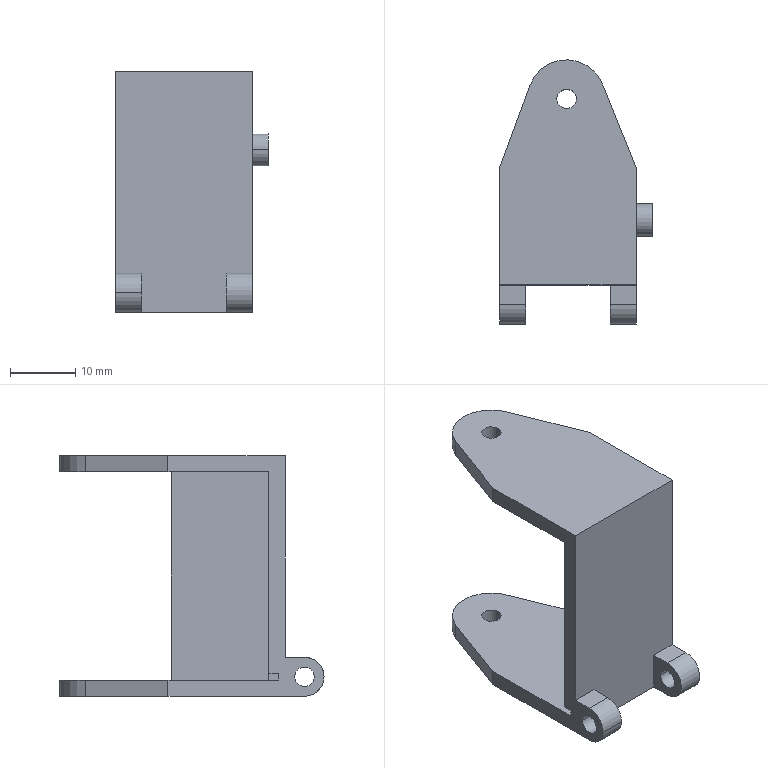Part | SolidWorks | features BaseBody 1 | 1 solid | 37 faces | box 23.5 x 40.616 x 37 mm | volume 6167 mm3 | plane 21 | cylinder 16 | commonest cylinder face diameters 3 x8 6 x3 5 x2 12 x2 8 x1
STEP:
#1=CARTESIAN_POINT('',(23.5,12.5,25.));
#2=VERTEX_POINT('',#1);
#3=CARTESIAN_POINT('',(23.5,7.5,25.));
#4=VERTEX_POINT('',#3);
#5=CARTESIAN_POINT('',(23.5,10.,25.));
#6=DIRECTION('',(1.,0.,0.));
#7=DIRECTION('',(0.,1.,0.));
#8=AXIS2_PLACEMENT_3D('',#5,#6,#7);
#9=CIRCLE('',#8,2.5);
#10=EDGE_CURVE('',#2,#4,#9,.T.);
#11=ORIENTED_EDGE('',*,*,#10,.F.);
#12=CARTESIAN_POINT('',(21.,12.5,25.));
#13=VERTEX_POINT('',#12);
#14=CARTESIAN_POINT('',(23.5,12.5,25.));
#15=DIRECTION('',(-1.,0.,0.));
#16=VECTOR('',#15,1000.);
#17=LINE('',#14,#16);
#18=EDGE_CURVE('',#2,#13,#17,.T.);
#19=ORIENTED_EDGE('',*,*,#18,.T.);
#20=CARTESIAN_POINT('',(21.,7.5,25.));
#21=VERTEX_POINT('',#20);
#22=CARTESIAN_POINT('',(21.,10.,25.));
#23=DIRECTION('',(1.,0.,0.));
#24=DIRECTION('',(0.,-1.,0.));
#25=AXIS2_PLACEMENT_3D('',#22,#23,#24);
#26=CIRCLE('',#25,2.5);
#27=EDGE_CURVE('',#13,#21,#26,.T.);
#28=ORIENTED_EDGE('',*,*,#27,.T.);
#29=CARTESIAN_POINT('',(23.5,7.5,25.));
#30=DIRECTION('',(-1.,0.,0.));
#31=VECTOR('',#30,1000.);
#32=LINE('',#29,#31);
#33=EDGE_CURVE('',#4,#21,#32,.T.);
#34=ORIENTED_EDGE('',*,*,#33,.F.);
#35=EDGE_LOOP('',(#11,#19,#28,#34));
#36=FACE_OUTER_BOUND('',#35,.T.);
#37=CARTESIAN_POINT('',(23.5,10.,25.));
#38=DIRECTION('',(-1.,0.,0.));
#39=DIRECTION('',(0.,-1.,0.));
#40=AXIS2_PLACEMENT_3D('',#37,#38,#39);
#41=CYLINDRICAL_SURFACE('',#40,2.5);
#42=ADVANCED_FACE('',(#36),#41,.T.);
#43=CARTESIAN_POINT('',(8.795,28.616,37.));
#44=VERTEX_POINT('',#43);
#45=CARTESIAN_POINT('',(11.795,28.616,37.));
#46=VERTEX_POINT('',#45);
#47=CARTESIAN_POINT('',(10.295,28.616,37.));
#48=DIRECTION('',(0.,0.,1.));
#49=DIRECTION('',(1.,0.,0.));
#50=AXIS2_PLACEMENT_3D('',#47,#48,#49);
#51=CIRCLE('',#50,1.5);
#52=EDGE_CURVE('',#44,#46,#51,.T.);
#53=ORIENTED_EDGE('',*,*,#52,.T.);
#54=CARTESIAN_POINT('',(11.795,28.616,34.5));
#55=VERTEX_POINT('',#54);
#56=CARTESIAN_POINT('',(11.795,28.616,43.));
#57=DIRECTION('',(0.,0.,-1.));
#58=VECTOR('',#57,1000.);
#59=LINE('',#56,#58);
#60=EDGE_CURVE('',#46,#55,#59,.T.);
#61=ORIENTED_EDGE('',*,*,#60,.T.);
#62=CARTESIAN_POINT('',(8.795,28.616,34.5));
#63=VERTEX_POINT('',#62);
#64=CARTESIAN_POINT('',(10.295,28.616,34.5));
#65=DIRECTION('',(0.,0.,1.));
#66=DIRECTION('',(1.,0.,0.));
#67=AXIS2_PLACEMENT_3D('',#64,#65,#66);
#68=CIRCLE('',#67,1.5);
#69=EDGE_CURVE('',#63,#55,#68,.T.);
#70=ORIENTED_EDGE('',*,*,#69,.F.);
#71=CARTESIAN_POINT('',(8.795,28.616,43.));
#72=DIRECTION('',(0.,0.,-1.));
#73=VECTOR('',#72,1000.);
#74=LINE('',#71,#73);
#75=EDGE_CURVE('',#44,#63,#74,.T.);
#76=ORIENTED_EDGE('',*,*,#75,.F.);
#77=EDGE_LOOP('',(#53,#61,#70,#76));
#78=FACE_OUTER_BOUND('',#77,.T.);
#79=CARTESIAN_POINT('',(10.295,28.616,43.));
#80=DIRECTION('',(0.,0.,-1.));
#81=DIRECTION('',(-1.,0.,0.));
#82=AXIS2_PLACEMENT_3D('',#79,#80,#81);
#83=CYLINDRICAL_SURFACE('',#82,1.5);
#84=ADVANCED_FACE('',(#78),#83,.F.);
#85=CARTESIAN_POINT('',(8.795,28.616,2.5));
#86=VERTEX_POINT('',#85);
#87=CARTESIAN_POINT('',(11.795,28.616,2.5));
#88=VERTEX_POINT('',#87);
#89=CARTESIAN_POINT('',(10.295,28.616,2.5));
#90=DIRECTION('',(0.,0.,1.));
#91=DIRECTION('',(1.,0.,0.));
#92=AXIS2_PLACEMENT_3D('',#89,#90,#91);
#93=CIRCLE('',#92,1.5);
#94=EDGE_CURVE('',#86,#88,#93,.T.);
#95=ORIENTED_EDGE('',*,*,#94,.T.);
#96=CARTESIAN_POINT('',(11.795,28.616,0.));
#97=VERTEX_POINT('',#96);
#98=CARTESIAN_POINT('',(11.795,28.616,43.));
#99=DIRECTION('',(0.,0.,-1.));
#100=VECTOR('',#99,1000.);
#101=LINE('',#98,#100);
#102=EDGE_CURVE('',#88,#97,#101,.T.);
#103=ORIENTED_EDGE('',*,*,#102,.T.);
#104=CARTESIAN_POINT('',(8.795,28.616,0.));
#105=VERTEX_POINT('',#104);
#106=CARTESIAN_POINT('',(10.295,28.616,0.));
#107=DIRECTION('',(0.,0.,-1.));
#108=DIRECTION('',(-1.,0.,0.));
#109=AXIS2_PLACEMENT_3D('',#106,#107,#108);
#110=CIRCLE('',#109,1.5);
#111=EDGE_CURVE('',#97,#105,#110,.T.);
#112=ORIENTED_EDGE('',*,*,#111,.T.);
#113=CARTESIAN_POINT('',(8.795,28.616,43.));
#114=DIRECTION('',(0.,0.,-1.));
#115=VECTOR('',#114,1000.);
#116=LINE('',#113,#115);
#117=EDGE_CURVE('',#86,#105,#116,.T.);
#118=ORIENTED_EDGE('',*,*,#117,.F.);
#119=EDGE_LOOP('',(#95,#103,#112,#118));
#120=FACE_OUTER_BOUND('',#119,.T.);
#121=CARTESIAN_POINT('',(10.295,28.616,43.));
#122=DIRECTION('',(0.,0.,-1.));
#123=DIRECTION('',(-1.,0.,0.));
#124=AXIS2_PLACEMENT_3D('',#121,#122,#123);
#125=CYLINDRICAL_SURFACE('',#124,1.5);
#126=ADVANCED_FACE('',(#120),#125,.F.);
#127=CARTESIAN_POINT('',(17.,-1.5,3.));
#128=VERTEX_POINT('',#127);
#129=CARTESIAN_POINT('',(17.,-4.5,3.));
#130=VERTEX_POINT('',#129);
#131=CARTESIAN_POINT('',(17.,-3.,3.));
#132=DIRECTION('',(-1.,0.,0.));
#133=DIRECTION('',(0.,-1.,0.));
#134=AXIS2_PLACEMENT_3D('',#131,#132,#133);
#135=CIRCLE('',#134,1.5);
#136=EDGE_CURVE('',#128,#130,#135,.T.);
#137=ORIENTED_EDGE('',*,*,#136,.T.);
#138=CARTESIAN_POINT('',(21.,-4.5,3.));
#139=VERTEX_POINT('',#138);
#140=CARTESIAN_POINT('',(17.,-4.5,3.));
#141=DIRECTION('',(1.,0.,0.));
#142=VECTOR('',#141,1000.);
#143=LINE('',#140,#142);
#144=EDGE_CURVE('',#130,#139,#143,.T.);
#145=ORIENTED_EDGE('',*,*,#144,.T.);
#146=CARTESIAN_POINT('',(21.,-1.5,3.));
#147=VERTEX_POINT('',#146);
#148=CARTESIAN_POINT('',(21.,-3.,3.));
#149=DIRECTION('',(-1.,0.,0.));
#150=DIRECTION('',(0.,-1.,0.));
#151=AXIS2_PLACEMENT_3D('',#148,#149,#150);
#152=CIRCLE('',#151,1.5);
#153=EDGE_CURVE('',#147,#139,#152,.T.);
#154=ORIENTED_EDGE('',*,*,#153,.F.);
#155=CARTESIAN_POINT('',(17.,-1.5,3.));
#156=DIRECTION('',(1.,0.,0.));
#157=VECTOR('',#156,1000.);
#158=LINE('',#155,#157);
#159=EDGE_CURVE('',#128,#147,#158,.T.);
#160=ORIENTED_EDGE('',*,*,#159,.F.);
#161=EDGE_LOOP('',(#137,#145,#154,#160));
#162=FACE_OUTER_BOUND('',#161,.T.);
#163=CARTESIAN_POINT('',(17.,-3.,3.));
#164=DIRECTION('',(1.,0.,0.));
#165=DIRECTION('',(0.,1.,0.));
#166=AXIS2_PLACEMENT_3D('',#163,#164,#165);
#167=CYLINDRICAL_SURFACE('',#166,1.5);
#168=ADVANCED_FACE('',(#162),#167,.F.);
#169=CARTESIAN_POINT('',(4.,-1.5,3.));
#170=VERTEX_POINT('',#169);
#171=CARTESIAN_POINT('',(4.,-4.5,3.));
#172=VERTEX_POINT('',#171);
#173=CARTESIAN_POINT('',(4.,-3.,3.));
#174=DIRECTION('',(-1.,0.,0.));
#175=DIRECTION('',(0.,-1.,0.));
#176=AXIS2_PLACEMENT_3D('',#173,#174,#175);
#177=CIRCLE('',#176,1.5);
#178=EDGE_CURVE('',#170,#172,#177,.T.);
#179=ORIENTED_EDGE('',*,*,#178,.F.);
#180=CARTESIAN_POINT('',(0.,-1.5,3.));
#181=VERTEX_POINT('',#180);
#182=CARTESIAN_POINT('',(4.,-1.5,3.));
#183=DIRECTION('',(-1.,0.,0.));
#184=VECTOR('',#183,1000.);
#185=LINE('',#182,#184);
#186=EDGE_CURVE('',#170,#181,#185,.T.);
#187=ORIENTED_EDGE('',*,*,#186,.T.);
#188=CARTESIAN_POINT('',(0.,-4.5,3.));
#189=VERTEX_POINT('',#188);
#190=CARTESIAN_POINT('',(0.,-3.,3.));
#191=DIRECTION('',(-1.,0.,0.));
#192=DIRECTION('',(0.,-1.,0.));
#193=AXIS2_PLACEMENT_3D('',#190,#191,#192);
#194=CIRCLE('',#193,1.5);
#195=EDGE_CURVE('',#181,#189,#194,.T.);
#196=ORIENTED_EDGE('',*,*,#195,.T.);
#197=CARTESIAN_POINT('',(4.,-4.5,3.));
#198=DIRECTION('',(-1.,0.,0.));
#199=VECTOR('',#198,1000.);
#200=LINE('',#197,#199);
#201=EDGE_CURVE('',#172,#189,#200,.T.);
#202=ORIENTED_EDGE('',*,*,#201,.F.);
#203=EDGE_LOOP('',(#179,#187,#196,#202));
#204=FACE_OUTER_BOUND('',#203,.T.);
#205=CARTESIAN_POINT('',(4.,-3.,3.));
#206=DIRECTION('',(-1.,0.,0.));
#207=DIRECTION('',(0.,-1.,0.));
#208=AXIS2_PLACEMENT_3D('',#205,#206,#207);
#209=CYLINDRICAL_SURFACE('',#208,1.5);
#210=ADVANCED_FACE('',(#204),#209,.F.);
#211=CARTESIAN_POINT('',(4.,-3.,0.));
#212=VERTEX_POINT('',#211);
#213=CARTESIAN_POINT('',(4.,-6.,3.));
#214=VERTEX_POINT('',#213);
#215=CARTESIAN_POINT('',(4.,-3.,3.));
#216=DIRECTION('',(-1.,0.,0.));
#217=DIRECTION('',(0.,-1.,0.));
#218=AXIS2_PLACEMENT_3D('',#215,#216,#217);
#219=CIRCLE('',#218,3.);
#220=EDGE_CURVE('',#212,#214,#219,.T.);
#221=ORIENTED_EDGE('',*,*,#220,.T.);
#222=CARTESIAN_POINT('',(0.,-6.,3.));
#223=VERTEX_POINT('',#222);
#224=CARTESIAN_POINT('',(4.,-6.,3.));
#225=DIRECTION('',(-1.,0.,0.));
#226=VECTOR('',#225,1000.);
#227=LINE('',#224,#226);
#228=EDGE_CURVE('',#214,#223,#227,.T.);
#229=ORIENTED_EDGE('',*,*,#228,.T.);
#230=CARTESIAN_POINT('',(0.,-3.,0.));
#231=VERTEX_POINT('',#230);
#232=CARTESIAN_POINT('',(0.,-3.,3.));
#233=DIRECTION('',(-1.,0.,0.));
#234=DIRECTION('',(0.,-1.,0.));
#235=AXIS2_PLACEMENT_3D('',#232,#233,#234);
#236=CIRCLE('',#235,3.);
#237=EDGE_CURVE('',#231,#223,#236,.T.);
#238=ORIENTED_EDGE('',*,*,#237,.F.);
#239=CARTESIAN_POINT('',(4.,-3.,0.));
#240=DIRECTION('',(-1.,0.,0.));
#241=VECTOR('',#240,1000.);
#242=LINE('',#239,#241);
#243=EDGE_CURVE('',#212,#231,#242,.T.);
#244=ORIENTED_EDGE('',*,*,#243,.F.);
#245=EDGE_LOOP('',(#221,#229,#238,#244));
#246=FACE_OUTER_BOUND('',#245,.T.);
#247=CARTESIAN_POINT('',(4.,-3.,3.));
#248=DIRECTION('',(-1.,0.,0.));
#249=DIRECTION('',(0.,-1.,0.));
#250=AXIS2_PLACEMENT_3D('',#247,#248,#249);
#251=CYLINDRICAL_SURFACE('',#250,3.);
#252=ADVANCED_FACE('',(#246),#251,.T.);
#253=CARTESIAN_POINT('',(16.029,30.384,2.5));
#254=VERTEX_POINT('',#253);
#255=CARTESIAN_POINT('',(16.029,30.384,0.));
#256=VERTEX_POINT('',#255);
#257=CARTESIAN_POINT('',(16.029,30.384,37.));
#258=DIRECTION('',(0.,0.,-1.));
#259=VECTOR('',#258,1000.);
#260=LINE('',#257,#259);
#261=EDGE_CURVE('',#254,#256,#260,.T.);
#262=ORIENTED_EDGE('',*,*,#261,.F.);
#263=CARTESIAN_POINT('',(21.,18.,2.5));
#264=VERTEX_POINT('',#263);
#265=CARTESIAN_POINT('',(21.,18.,2.5));
#266=DIRECTION('',(0.3725,-0.928,0.));
#267=VECTOR('',#266,1000.);
#268=LINE('',#265,#267);
#269=EDGE_CURVE('',#254,#264,#268,.T.);
#270=ORIENTED_EDGE('',*,*,#269,.T.);
#271=CARTESIAN_POINT('',(21.,18.,0.));
#272=VERTEX_POINT('',#271);
#273=CARTESIAN_POINT('',(21.,18.,37.));
#274=DIRECTION('',(0.,0.,-1.));
#275=VECTOR('',#274,1000.);
#276=LINE('',#273,#275);
#277=EDGE_CURVE('',#264,#272,#276,.T.);
#278=ORIENTED_EDGE('',*,*,#277,.T.);
#279=CARTESIAN_POINT('',(21.,18.,0.));
#280=DIRECTION('',(-0.3725,0.928,0.));
#281=VECTOR('',#280,1000.);
#282=LINE('',#279,#281);
#283=EDGE_CURVE('',#272,#256,#282,.T.);
#284=ORIENTED_EDGE('',*,*,#283,.T.);
#285=EDGE_LOOP('',(#262,#270,#278,#284));
#286=FACE_OUTER_BOUND('',#285,.T.);
#287=CARTESIAN_POINT('',(21.,18.,37.));
#288=DIRECTION('',(-0.928,-0.3725,0.));
#289=DIRECTION('',(0.3725,-0.928,0.));
#290=AXIS2_PLACEMENT_3D('',#287,#288,#289);
#291=PLANE('',#290);
#292=ADVANCED_FACE('',(#286),#291,.F.);
#293=CARTESIAN_POINT('',(4.663,30.686,2.5));
#294=VERTEX_POINT('',#293);
#295=CARTESIAN_POINT('',(10.295,28.616,2.5));
#296=DIRECTION('',(0.,0.,1.));
#297=DIRECTION('',(1.,0.,0.));
#298=AXIS2_PLACEMENT_3D('',#295,#296,#297);
#299=CIRCLE('',#298,6.);
#300=EDGE_CURVE('',#254,#294,#299,.T.);
#301=ORIENTED_EDGE('',*,*,#300,.F.);
#302=ORIENTED_EDGE('',*,*,#261,.T.);
#303=CARTESIAN_POINT('',(4.663,30.686,0.));
#304=VERTEX_POINT('',#303);
#305=CARTESIAN_POINT('',(10.295,28.616,0.));
#306=DIRECTION('',(0.,0.,1.));
#307=DIRECTION('',(1.,0.,0.));
#308=AXIS2_PLACEMENT_3D('',#305,#306,#307);
#309=CIRCLE('',#308,6.);
#310=EDGE_CURVE('',#256,#304,#309,.T.);
#311=ORIENTED_EDGE('',*,*,#310,.T.);
#312=CARTESIAN_POINT('',(4.663,30.686,37.));
#313=DIRECTION('',(0.,0.,-1.));
#314=VECTOR('',#313,1000.);
#315=LINE('',#312,#314);
#316=EDGE_CURVE('',#294,#304,#315,.T.);
#317=ORIENTED_EDGE('',*,*,#316,.F.);
#318=EDGE_LOOP('',(#301,#302,#311,#317));
#319=FACE_OUTER_BOUND('',#318,.T.);
#320=CARTESIAN_POINT('',(10.295,28.616,37.));
#321=DIRECTION('',(0.,0.,-1.));
#322=DIRECTION('',(-1.,0.,0.));
#323=AXIS2_PLACEMENT_3D('',#320,#321,#322);
#324=CYLINDRICAL_SURFACE('',#323,6.);
#325=ADVANCED_FACE('',(#319),#324,.T.);
#326=CARTESIAN_POINT('',(0.,18.,2.5));
#327=VERTEX_POINT('',#326);
#328=CARTESIAN_POINT('',(4.663,30.686,2.5));
#329=DIRECTION('',(-0.345,-0.9386,0.));
#330=VECTOR('',#329,1000.);
#331=LINE('',#328,#330);
#332=EDGE_CURVE('',#294,#327,#331,.T.);
#333=ORIENTED_EDGE('',*,*,#332,.F.);
#334=ORIENTED_EDGE('',*,*,#316,.T.);
#335=CARTESIAN_POINT('',(0.,18.,0.));
#336=VERTEX_POINT('',#335);
#337=CARTESIAN_POINT('',(4.663,30.686,0.));
#338=DIRECTION('',(-0.345,-0.9386,0.));
#339=VECTOR('',#338,1000.);
#340=LINE('',#337,#339);
#341=EDGE_CURVE('',#304,#336,#340,.T.);
#342=ORIENTED_EDGE('',*,*,#341,.T.);
#343=CARTESIAN_POINT('',(0.,18.,37.));
#344=DIRECTION('',(0.,0.,-1.));
#345=VECTOR('',#344,1000.);
#346=LINE('',#343,#345);
#347=EDGE_CURVE('',#327,#336,#346,.T.);
#348=ORIENTED_EDGE('',*,*,#347,.F.);
#349=EDGE_LOOP('',(#333,#334,#342,#348));
#350=FACE_OUTER_BOUND('',#349,.T.);
#351=CARTESIAN_POINT('',(4.663,30.686,37.));
#352=DIRECTION('',(0.9386,-0.345,0.));
#353=DIRECTION('',(0.345,0.9386,0.));
#354=AXIS2_PLACEMENT_3D('',#351,#352,#353);
#355=PLANE('',#354);
#356=ADVANCED_FACE('',(#350),#355,.F.);
#357=CARTESIAN_POINT('',(0.,-3.,3.));
#358=DIRECTION('',(-1.,0.,0.));
#359=DIRECTION('',(0.,-1.,0.));
#360=AXIS2_PLACEMENT_3D('',#357,#358,#359);
#361=CIRCLE('',#360,1.5);
#362=EDGE_CURVE('',#189,#181,#361,.T.);
#363=ORIENTED_EDGE('',*,*,#362,.F.);
#364=ORIENTED_EDGE('',*,*,#195,.F.);
#365=EDGE_LOOP('',(#363,#364));
#366=FACE_BOUND('',#365,.T.);
#367=CARTESIAN_POINT('',(0.,0.9686,2.5));
#368=VERTEX_POINT('',#367);
#369=CARTESIAN_POINT('',(0.,18.,2.5));
#370=DIRECTION('',(0.,-1.,0.));
#371=VECTOR('',#370,1000.);
#372=LINE('',#369,#371);
#373=EDGE_CURVE('',#327,#368,#372,.T.);
#374=ORIENTED_EDGE('',*,*,#373,.F.);
#375=ORIENTED_EDGE('',*,*,#347,.T.);
#376=CARTESIAN_POINT('',(0.,18.,0.));
#377=DIRECTION('',(0.,-1.,0.));
#378=VECTOR('',#377,1000.);
#379=LINE('',#376,#378);
#380=EDGE_CURVE('',#336,#231,#379,.T.);
#381=ORIENTED_EDGE('',*,*,#380,.T.);
#382=ORIENTED_EDGE('',*,*,#237,.T.);
#383=CARTESIAN_POINT('',(0.,-3.,6.));
#384=VERTEX_POINT('',#383);
#385=CARTESIAN_POINT('',(0.,-3.,3.));
#386=DIRECTION('',(-1.,0.,0.));
#387=DIRECTION('',(0.,-1.,0.));
#388=AXIS2_PLACEMENT_3D('',#385,#386,#387);
#389=CIRCLE('',#388,3.);
#390=EDGE_CURVE('',#223,#384,#389,.T.);
#391=ORIENTED_EDGE('',*,*,#390,.T.);
#392=CARTESIAN_POINT('',(0.,0.,6.));
#393=VERTEX_POINT('',#392);
#394=CARTESIAN_POINT('',(0.,-3.,6.));
#395=DIRECTION('',(0.,1.,0.));
#396=VECTOR('',#395,1000.);
#397=LINE('',#394,#396);
#398=EDGE_CURVE('',#384,#393,#397,.T.);
#399=ORIENTED_EDGE('',*,*,#398,.T.);
#400=CARTESIAN_POINT('',(0.,0.,37.));
#401=VERTEX_POINT('',#400);
#402=CARTESIAN_POINT('',(0.,0.,37.));
#403=DIRECTION('',(0.,0.,-1.));
#404=VECTOR('',#403,1000.);
#405=LINE('',#402,#404);
#406=EDGE_CURVE('',#401,#393,#405,.T.);
#407=ORIENTED_EDGE('',*,*,#406,.F.);
#408=CARTESIAN_POINT('',(0.,18.,37.));
#409=VERTEX_POINT('',#408);
#410=CARTESIAN_POINT('',(0.,18.,37.));
#411=DIRECTION('',(0.,-1.,0.));
#412=VECTOR('',#411,1000.);
#413=LINE('',#410,#412);
#414=EDGE_CURVE('',#409,#401,#413,.T.);
#415=ORIENTED_EDGE('',*,*,#414,.F.);
#416=CARTESIAN_POINT('',(0.,18.,34.5));
#417=VERTEX_POINT('',#416);
#418=CARTESIAN_POINT('',(0.,18.,37.));
#419=DIRECTION('',(0.,0.,-1.));
#420=VECTOR('',#419,1000.);
#421=LINE('',#418,#420);
#422=EDGE_CURVE('',#409,#417,#421,.T.);
#423=ORIENTED_EDGE('',*,*,#422,.T.);
#424=CARTESIAN_POINT('',(0.,2.5,34.5));
#425=VERTEX_POINT('',#424);
#426=CARTESIAN_POINT('',(0.,18.,34.5));
#427=DIRECTION('',(0.,-1.,0.));
#428=VECTOR('',#427,1000.);
#429=LINE('',#426,#428);
#430=EDGE_CURVE('',#417,#425,#429,.T.);
#431=ORIENTED_EDGE('',*,*,#430,.T.);
#432=CARTESIAN_POINT('',(0.,2.5,3.5));
#433=VERTEX_POINT('',#432);
#434=CARTESIAN_POINT('',(0.,2.5,37.));
#435=DIRECTION('',(0.,0.,-1.));
#436=VECTOR('',#435,1000.);
#437=LINE('',#434,#436);
#438=EDGE_CURVE('',#425,#433,#437,.T.);
#439=ORIENTED_EDGE('',*,*,#438,.T.);
#440=CARTESIAN_POINT('',(0.,0.9686,3.5));
#441=VERTEX_POINT('',#440);
#442=CARTESIAN_POINT('',(0.,-3.,3.5));
#443=DIRECTION('',(0.,1.,0.));
#444=VECTOR('',#443,1000.);
#445=LINE('',#442,#444);
#446=EDGE_CURVE('',#441,#433,#445,.T.);
#447=ORIENTED_EDGE('',*,*,#446,.F.);
#448=CARTESIAN_POINT('',(0.,-3.,3.));
#449=DIRECTION('',(-1.,0.,0.));
#450=DIRECTION('',(0.,1.,0.));
#451=AXIS2_PLACEMENT_3D('',#448,#449,#450);
#452=CIRCLE('',#451,4.);
#453=EDGE_CURVE('',#441,#368,#452,.T.);
#454=ORIENTED_EDGE('',*,*,#453,.T.);
#455=EDGE_LOOP('',(#374,#375,#381,#382,#391,#399,#407,#415,#423,#431,#439,#447,#454));
#456=FACE_OUTER_BOUND('',#455,.T.);
#457=CARTESIAN_POINT('',(0.,18.,37.));
#458=DIRECTION('',(1.,0.,0.));
#459=DIRECTION('',(0.,1.,0.));
#460=AXIS2_PLACEMENT_3D('',#457,#458,#459);
#461=PLANE('',#460);
#462=ADVANCED_FACE('',(#366,#456),#461,.F.);
#463=CARTESIAN_POINT('',(17.,0.,6.));
#464=VERTEX_POINT('',#463);
#465=CARTESIAN_POINT('',(17.,0.,0.));
#466=VERTEX_POINT('',#465);
#467=CARTESIAN_POINT('',(17.,0.,6.));
#468=DIRECTION('',(0.,0.,-1.));
#469=VECTOR('',#468,1000.);
#470=LINE('',#467,#469);
#471=EDGE_CURVE('',#464,#466,#470,.T.);
#472=ORIENTED_EDGE('',*,*,#471,.F.);
#473=CARTESIAN_POINT('',(21.,0.,6.));
#474=VERTEX_POINT('',#473);
#475=CARTESIAN_POINT('',(17.,0.,6.));
#476=DIRECTION('',(1.,0.,0.));
#477=VECTOR('',#476,1000.);
#478=LINE('',#475,#477);
#479=EDGE_CURVE('',#464,#474,#478,.T.);
#480=ORIENTED_EDGE('',*,*,#479,.T.);
#481=CARTESIAN_POINT('',(21.,0.,37.));
#482=VERTEX_POINT('',#481);
#483=CARTESIAN_POINT('',(21.,0.,37.));
#484=DIRECTION('',(0.,0.,-1.));
#485=VECTOR('',#484,1000.);
#486=LINE('',#483,#485);
#487=EDGE_CURVE('',#482,#474,#486,.T.);
#488=ORIENTED_EDGE('',*,*,#487,.F.);
#489=CARTESIAN_POINT('',(0.,0.,37.));
#490=DIRECTION('',(1.,0.,0.));
#491=VECTOR('',#490,1000.);
#492=LINE('',#489,#491);
#493=EDGE_CURVE('',#401,#482,#492,.T.);
#494=ORIENTED_EDGE('',*,*,#493,.F.);
#495=ORIENTED_EDGE('',*,*,#406,.T.);
#496=CARTESIAN_POINT('',(4.,0.,6.));
#497=VERTEX_POINT('',#496);
#498=CARTESIAN_POINT('',(4.,0.,6.));
#499=DIRECTION('',(-1.,0.,0.));
#500=VECTOR('',#499,1000.);
#501=LINE('',#498,#500);
#502=EDGE_CURVE('',#497,#393,#501,.T.);
#503=ORIENTED_EDGE('',*,*,#502,.F.);
#504=CARTESIAN_POINT('',(4.,0.,0.));
#505=VERTEX_POINT('',#504);
#506=CARTESIAN_POINT('',(4.,0.,6.));
#507=DIRECTION('',(0.,0.,-1.));
#508=VECTOR('',#507,1000.);
#509=LINE('',#506,#508);
#510=EDGE_CURVE('',#497,#505,#509,.T.);
#511=ORIENTED_EDGE('',*,*,#510,.T.);
#512=CARTESIAN_POINT('',(0.,0.,0.));
#513=DIRECTION('',(1.,0.,0.));
#514=VECTOR('',#513,1000.);
#515=LINE('',#512,#514);
#516=EDGE_CURVE('',#505,#466,#515,.T.);
#517=ORIENTED_EDGE('',*,*,#516,.T.);
#518=EDGE_LOOP('',(#472,#480,#488,#494,#495,#503,#511,#517));
#519=FACE_OUTER_BOUND('',#518,.T.);
#520=CARTESIAN_POINT('',(0.,0.,37.));
#521=DIRECTION('',(0.,1.,0.));
#522=DIRECTION('',(0.,0.,1.));
#523=AXIS2_PLACEMENT_3D('',#520,#521,#522);
#524=PLANE('',#523);
#525=ADVANCED_FACE('',(#519),#524,.F.);
#526=CARTESIAN_POINT('',(21.,10.,25.));
#527=DIRECTION('',(1.,0.,0.));
#528=DIRECTION('',(0.,-1.,0.));
#529=AXIS2_PLACEMENT_3D('',#526,#527,#528);
#530=CIRCLE('',#529,2.5);
#531=EDGE_CURVE('',#21,#13,#530,.T.);
#532=ORIENTED_EDGE('',*,*,#531,.F.);
#533=ORIENTED_EDGE('',*,*,#27,.F.);
#534=EDGE_LOOP('',(#532,#533));
#535=FACE_BOUND('',#534,.T.);
#536=ORIENTED_EDGE('',*,*,#277,.F.);
#537=CARTESIAN_POINT('',(21.,17.517,2.5));
#538=VERTEX_POINT('',#537);
#539=CARTESIAN_POINT('',(21.,0.,2.5));
#540=DIRECTION('',(0.,-1.,0.));
#541=VECTOR('',#540,1000.);
#542=LINE('',#539,#541);
#543=EDGE_CURVE('',#264,#538,#542,.T.);
#544=ORIENTED_EDGE('',*,*,#543,.T.);
#545=CARTESIAN_POINT('',(21.,17.517,34.5));
#546=VERTEX_POINT('',#545);
#547=CARTESIAN_POINT('',(21.,17.517,37.));
#548=DIRECTION('',(0.,0.,1.));
#549=VECTOR('',#548,1000.);
#550=LINE('',#547,#549);
#551=EDGE_CURVE('',#538,#546,#550,.T.);
#552=ORIENTED_EDGE('',*,*,#551,.T.);
#553=CARTESIAN_POINT('',(21.,18.,34.5));
#554=VERTEX_POINT('',#553);
#555=CARTESIAN_POINT('',(21.,0.,34.5));
#556=DIRECTION('',(0.,1.,0.));
#557=VECTOR('',#556,1000.);
#558=LINE('',#555,#557);
#559=EDGE_CURVE('',#546,#554,#558,.T.);
#560=ORIENTED_EDGE('',*,*,#559,.T.);
#561=CARTESIAN_POINT('',(21.,18.,37.));
#562=VERTEX_POINT('',#561);
#563=CARTESIAN_POINT('',(21.,18.,37.));
#564=DIRECTION('',(0.,0.,-1.));
#565=VECTOR('',#564,1000.);
#566=LINE('',#563,#565);
#567=EDGE_CURVE('',#562,#554,#566,.T.);
#568=ORIENTED_EDGE('',*,*,#567,.F.);
#569=CARTESIAN_POINT('',(21.,0.,37.));
#570=DIRECTION('',(0.,1.,0.));
#571=VECTOR('',#570,1000.);
#572=LINE('',#569,#571);
#573=EDGE_CURVE('',#482,#562,#572,.T.);
#574=ORIENTED_EDGE('',*,*,#573,.F.);
#575=ORIENTED_EDGE('',*,*,#487,.T.);
#576=CARTESIAN_POINT('',(21.,-3.,6.));
#577=VERTEX_POINT('',#576);
#578=CARTESIAN_POINT('',(21.,-3.,6.));
#579=DIRECTION('',(0.,1.,0.));
#580=VECTOR('',#579,1000.);
#581=LINE('',#578,#580);
#582=EDGE_CURVE('',#577,#474,#581,.T.);
#583=ORIENTED_EDGE('',*,*,#582,.F.);
#584=CARTESIAN_POINT('',(21.,-3.,0.));
#585=VERTEX_POINT('',#584);
#586=CARTESIAN_POINT('',(21.,-3.,3.));
#587=DIRECTION('',(-1.,0.,0.));
#588=DIRECTION('',(0.,-1.,0.));
#589=AXIS2_PLACEMENT_3D('',#586,#587,#588);
#590=CIRCLE('',#589,3.);
#591=EDGE_CURVE('',#585,#577,#590,.T.);
#592=ORIENTED_EDGE('',*,*,#591,.F.);
#593=CARTESIAN_POINT('',(21.,0.,0.));
#594=DIRECTION('',(0.,1.,0.));
#595=VECTOR('',#594,1000.);
#596=LINE('',#593,#595);
#597=EDGE_CURVE('',#585,#272,#596,.T.);
#598=ORIENTED_EDGE('',*,*,#597,.T.);
#599=EDGE_LOOP('',(#536,#544,#552,#560,#568,#574,#575,#583,#592,#598));
#600=FACE_OUTER_BOUND('',#599,.T.);
#601=ORIENTED_EDGE('',*,*,#153,.T.);
#602=CARTESIAN_POINT('',(21.,-3.,3.));
#603=DIRECTION('',(-1.,0.,0.));
#604=DIRECTION('',(0.,-1.,0.));
#605=AXIS2_PLACEMENT_3D('',#602,#603,#604);
#606=CIRCLE('',#605,1.5);
#607=EDGE_CURVE('',#139,#147,#606,.T.);
#608=ORIENTED_EDGE('',*,*,#607,.T.);
#609=EDGE_LOOP('',(#601,#608));
#610=FACE_BOUND('',#609,.T.);
#611=CARTESIAN_POINT('',(21.,0.,37.));
#612=DIRECTION('',(-1.,0.,0.));
#613=DIRECTION('',(0.,-1.,0.));
#614=AXIS2_PLACEMENT_3D('',#611,#612,#613);
#615=PLANE('',#614);
#616=ADVANCED_FACE('',(#535,#600,#610),#615,.F.);
#617=ORIENTED_EDGE('',*,*,#567,.T.);
#618=CARTESIAN_POINT('',(16.029,30.384,34.5));
#619=VERTEX_POINT('',#618);
#620=CARTESIAN_POINT('',(21.,18.,34.5));
#621=DIRECTION('',(-0.3725,0.928,0.));
#622=VECTOR('',#621,1000.);
#623=LINE('',#620,#622);
#624=EDGE_CURVE('',#554,#619,#623,.T.);
#625=ORIENTED_EDGE('',*,*,#624,.T.);
#626=CARTESIAN_POINT('',(16.029,30.384,37.));
#627=VERTEX_POINT('',#626);
#628=CARTESIAN_POINT('',(16.029,30.384,37.));
#629=DIRECTION('',(0.,0.,-1.));
#630=VECTOR('',#629,1000.);
#631=LINE('',#628,#630);
#632=EDGE_CURVE('',#627,#619,#631,.T.);
#633=ORIENTED_EDGE('',*,*,#632,.F.);
#634=CARTESIAN_POINT('',(21.,18.,37.));
#635=DIRECTION('',(-0.3725,0.928,0.));
#636=VECTOR('',#635,1000.);
#637=LINE('',#634,#636);
#638=EDGE_CURVE('',#562,#627,#637,.T.);
#639=ORIENTED_EDGE('',*,*,#638,.F.);
#640=EDGE_LOOP('',(#617,#625,#633,#639));
#641=FACE_OUTER_BOUND('',#640,.T.);
#642=CARTESIAN_POINT('',(21.,18.,37.));
#643=DIRECTION('',(-0.928,-0.3725,0.));
#644=DIRECTION('',(0.3725,-0.928,0.));
#645=AXIS2_PLACEMENT_3D('',#642,#643,#644);
#646=PLANE('',#645);
#647=ADVANCED_FACE('',(#641),#646,.F.);
#648=ORIENTED_EDGE('',*,*,#632,.T.);
#649=CARTESIAN_POINT('',(4.663,30.686,34.5));
#650=VERTEX_POINT('',#649);
#651=CARTESIAN_POINT('',(10.295,28.616,34.5));
#652=DIRECTION('',(0.,0.,1.));
#653=DIRECTION('',(1.,0.,0.));
#654=AXIS2_PLACEMENT_3D('',#651,#652,#653);
#655=CIRCLE('',#654,6.);
#656=EDGE_CURVE('',#619,#650,#655,.T.);
#657=ORIENTED_EDGE('',*,*,#656,.T.);
#658=CARTESIAN_POINT('',(4.663,30.686,37.));
#659=VERTEX_POINT('',#658);
#660=CARTESIAN_POINT('',(4.663,30.686,37.));
#661=DIRECTION('',(0.,0.,-1.));
#662=VECTOR('',#661,1000.);
#663=LINE('',#660,#662);
#664=EDGE_CURVE('',#659,#650,#663,.T.);
#665=ORIENTED_EDGE('',*,*,#664,.F.);
#666=CARTESIAN_POINT('',(10.295,28.616,37.));
#667=DIRECTION('',(0.,0.,1.));
#668=DIRECTION('',(1.,0.,0.));
#669=AXIS2_PLACEMENT_3D('',#666,#667,#668);
#670=CIRCLE('',#669,6.);
#671=EDGE_CURVE('',#627,#659,#670,.T.);
#672=ORIENTED_EDGE('',*,*,#671,.F.);
#673=EDGE_LOOP('',(#648,#657,#665,#672));
#674=FACE_OUTER_BOUND('',#673,.T.);
#675=CARTESIAN_POINT('',(10.295,28.616,37.));
#676=DIRECTION('',(0.,0.,-1.));
#677=DIRECTION('',(-1.,0.,0.));
#678=AXIS2_PLACEMENT_3D('',#675,#676,#677);
#679=CYLINDRICAL_SURFACE('',#678,6.);
#680=ADVANCED_FACE('',(#674),#679,.T.);
#681=ORIENTED_EDGE('',*,*,#664,.T.);
#682=CARTESIAN_POINT('',(4.663,30.686,34.5));
#683=DIRECTION('',(-0.345,-0.9386,0.));
#684=VECTOR('',#683,1000.);
#685=LINE('',#682,#684);
#686=EDGE_CURVE('',#650,#417,#685,.T.);
#687=ORIENTED_EDGE('',*,*,#686,.T.);
#688=ORIENTED_EDGE('',*,*,#422,.F.);
#689=CARTESIAN_POINT('',(4.663,30.686,37.));
#690=DIRECTION('',(-0.345,-0.9386,0.));
#691=VECTOR('',#690,1000.);
#692=LINE('',#689,#691);
#693=EDGE_CURVE('',#659,#409,#692,.T.);
#694=ORIENTED_EDGE('',*,*,#693,.F.);
#695=EDGE_LOOP('',(#681,#687,#688,#694));
#696=FACE_OUTER_BOUND('',#695,.T.);
#697=CARTESIAN_POINT('',(4.663,30.686,37.));
#698=DIRECTION('',(0.9386,-0.345,0.));
#699=DIRECTION('',(0.345,0.9386,0.));
#700=AXIS2_PLACEMENT_3D('',#697,#698,#699);
#701=PLANE('',#700);
#702=ADVANCED_FACE('',(#696),#701,.F.);
#703=ORIENTED_EDGE('',*,*,#52,.F.);
#704=CARTESIAN_POINT('',(10.295,28.616,37.));
#705=DIRECTION('',(0.,0.,1.));
#706=DIRECTION('',(1.,0.,0.));
#707=AXIS2_PLACEMENT_3D('',#704,#705,#706);
#708=CIRCLE('',#707,1.5);
#709=EDGE_CURVE('',#46,#44,#708,.T.);
#710=ORIENTED_EDGE('',*,*,#709,.F.);
#711=EDGE_LOOP('',(#703,#710));
#712=FACE_BOUND('',#711,.T.);
#713=ORIENTED_EDGE('',*,*,#493,.T.);
#714=ORIENTED_EDGE('',*,*,#573,.T.);
#715=ORIENTED_EDGE('',*,*,#638,.T.);
#716=ORIENTED_EDGE('',*,*,#671,.T.);
#717=ORIENTED_EDGE('',*,*,#693,.T.);
#718=ORIENTED_EDGE('',*,*,#414,.T.);
#719=EDGE_LOOP('',(#713,#714,#715,#716,#717,#718));
#720=FACE_OUTER_BOUND('',#719,.T.);
#721=CARTESIAN_POINT('',(10.295,28.616,37.));
#722=DIRECTION('',(0.,0.,1.));
#723=DIRECTION('',(1.,0.,0.));
#724=AXIS2_PLACEMENT_3D('',#721,#722,#723);
#725=PLANE('',#724);
#726=ADVANCED_FACE('',(#712,#720),#725,.T.);
#727=CARTESIAN_POINT('',(10.295,28.616,0.));
#728=DIRECTION('',(0.,0.,-1.));
#729=DIRECTION('',(-1.,0.,0.));
#730=AXIS2_PLACEMENT_3D('',#727,#728,#729);
#731=CIRCLE('',#730,1.5);
#732=EDGE_CURVE('',#105,#97,#731,.T.);
#733=ORIENTED_EDGE('',*,*,#732,.F.);
#734=ORIENTED_EDGE('',*,*,#111,.F.);
#735=EDGE_LOOP('',(#733,#734));
#736=FACE_BOUND('',#735,.T.);
#737=ORIENTED_EDGE('',*,*,#516,.F.);
#738=CARTESIAN_POINT('',(4.,0.,0.));
#739=DIRECTION('',(0.,-1.,0.));
#740=VECTOR('',#739,1000.);
#741=LINE('',#738,#740);
#742=EDGE_CURVE('',#505,#212,#741,.T.);
#743=ORIENTED_EDGE('',*,*,#742,.T.);
#744=ORIENTED_EDGE('',*,*,#243,.T.);
#745=ORIENTED_EDGE('',*,*,#380,.F.);
#746=ORIENTED_EDGE('',*,*,#341,.F.);
#747=ORIENTED_EDGE('',*,*,#310,.F.);
#748=ORIENTED_EDGE('',*,*,#283,.F.);
#749=ORIENTED_EDGE('',*,*,#597,.F.);
#750=CARTESIAN_POINT('',(17.,-3.,0.));
#751=VERTEX_POINT('',#750);
#752=CARTESIAN_POINT('',(17.,-3.,0.));
#753=DIRECTION('',(1.,0.,0.));
#754=VECTOR('',#753,1000.);
#755=LINE('',#752,#754);
#756=EDGE_CURVE('',#751,#585,#755,.T.);
#757=ORIENTED_EDGE('',*,*,#756,.F.);
#758=CARTESIAN_POINT('',(17.,0.,0.));
#759=DIRECTION('',(0.,-1.,0.));
#760=VECTOR('',#759,1000.);
#761=LINE('',#758,#760);
#762=EDGE_CURVE('',#466,#751,#761,.T.);
#763=ORIENTED_EDGE('',*,*,#762,.F.);
#764=EDGE_LOOP('',(#737,#743,#744,#745,#746,#747,#748,#749,#757,#763));
#765=FACE_OUTER_BOUND('',#764,.T.);
#766=CARTESIAN_POINT('',(10.295,28.616,0.));
#767=DIRECTION('',(0.,0.,1.));
#768=DIRECTION('',(1.,0.,0.));
#769=AXIS2_PLACEMENT_3D('',#766,#767,#768);
#770=PLANE('',#769);
#771=ADVANCED_FACE('',(#736,#765),#770,.F.);
#772=ORIENTED_EDGE('',*,*,#398,.F.);
#773=CARTESIAN_POINT('',(4.,-3.,6.));
#774=VERTEX_POINT('',#773);
#775=CARTESIAN_POINT('',(4.,-3.,6.));
#776=DIRECTION('',(-1.,0.,0.));
#777=VECTOR('',#776,1000.);
#778=LINE('',#775,#777);
#779=EDGE_CURVE('',#774,#384,#778,.T.);
#780=ORIENTED_EDGE('',*,*,#779,.F.);
#781=CARTESIAN_POINT('',(4.,-3.,6.));
#782=DIRECTION('',(0.,1.,0.));
#783=VECTOR('',#782,1000.);
#784=LINE('',#781,#783);
#785=EDGE_CURVE('',#774,#497,#784,.T.);
#786=ORIENTED_EDGE('',*,*,#785,.T.);
#787=ORIENTED_EDGE('',*,*,#502,.T.);
#788=EDGE_LOOP('',(#772,#780,#786,#787));
#789=FACE_OUTER_BOUND('',#788,.T.);
#790=CARTESIAN_POINT('',(4.,-3.,6.));
#791=DIRECTION('',(0.,0.,1.));
#792=DIRECTION('',(0.,-1.,0.));
#793=AXIS2_PLACEMENT_3D('',#790,#791,#792);
#794=PLANE('',#793);
#795=ADVANCED_FACE('',(#789),#794,.T.);
#796=ORIENTED_EDGE('',*,*,#228,.F.);
#797=CARTESIAN_POINT('',(4.,-3.,3.));
#798=DIRECTION('',(-1.,0.,0.));
#799=DIRECTION('',(0.,-1.,0.));
#800=AXIS2_PLACEMENT_3D('',#797,#798,#799);
#801=CIRCLE('',#800,3.);
#802=EDGE_CURVE('',#214,#774,#801,.T.);
#803=ORIENTED_EDGE('',*,*,#802,.T.);
#804=ORIENTED_EDGE('',*,*,#779,.T.);
#805=ORIENTED_EDGE('',*,*,#390,.F.);
#806=EDGE_LOOP('',(#796,#803,#804,#805));
#807=FACE_OUTER_BOUND('',#806,.T.);
#808=CARTESIAN_POINT('',(4.,-3.,3.));
#809=DIRECTION('',(-1.,0.,0.));
#810=DIRECTION('',(0.,-1.,0.));
#811=AXIS2_PLACEMENT_3D('',#808,#809,#810);
#812=CYLINDRICAL_SURFACE('',#811,3.);
#813=ADVANCED_FACE('',(#807),#812,.T.);
#814=CARTESIAN_POINT('',(4.,-3.,3.));
#815=DIRECTION('',(-1.,0.,0.));
#816=DIRECTION('',(0.,-1.,0.));
#817=AXIS2_PLACEMENT_3D('',#814,#815,#816);
#818=CIRCLE('',#817,1.5);
#819=EDGE_CURVE('',#172,#170,#818,.T.);
#820=ORIENTED_EDGE('',*,*,#819,.T.);
#821=ORIENTED_EDGE('',*,*,#178,.T.);
#822=EDGE_LOOP('',(#820,#821));
#823=FACE_BOUND('',#822,.T.);
#824=ORIENTED_EDGE('',*,*,#510,.F.);
#825=ORIENTED_EDGE('',*,*,#785,.F.);
#826=ORIENTED_EDGE('',*,*,#802,.F.);
#827=ORIENTED_EDGE('',*,*,#220,.F.);
#828=ORIENTED_EDGE('',*,*,#742,.F.);
#829=EDGE_LOOP('',(#824,#825,#826,#827,#828));
#830=FACE_OUTER_BOUND('',#829,.T.);
#831=CARTESIAN_POINT('',(4.,-3.,3.));
#832=DIRECTION('',(-1.,0.,0.));
#833=DIRECTION('',(0.,-1.,0.));
#834=AXIS2_PLACEMENT_3D('',#831,#832,#833);
#835=PLANE('',#834);
#836=ADVANCED_FACE('',(#823,#830),#835,.F.);
#837=ORIENTED_EDGE('',*,*,#186,.F.);
#838=ORIENTED_EDGE('',*,*,#819,.F.);
#839=ORIENTED_EDGE('',*,*,#201,.T.);
#840=ORIENTED_EDGE('',*,*,#362,.T.);
#841=EDGE_LOOP('',(#837,#838,#839,#840));
#842=FACE_OUTER_BOUND('',#841,.T.);
#843=CARTESIAN_POINT('',(4.,-3.,3.));
#844=DIRECTION('',(-1.,0.,0.));
#845=DIRECTION('',(0.,-1.,0.));
#846=AXIS2_PLACEMENT_3D('',#843,#844,#845);
#847=CYLINDRICAL_SURFACE('',#846,1.5);
#848=ADVANCED_FACE('',(#842),#847,.F.);
#849=ORIENTED_EDGE('',*,*,#471,.T.);
#850=ORIENTED_EDGE('',*,*,#762,.T.);
#851=CARTESIAN_POINT('',(17.,-3.,6.));
#852=VERTEX_POINT('',#851);
#853=CARTESIAN_POINT('',(17.,-3.,3.));
#854=DIRECTION('',(-1.,0.,0.));
#855=DIRECTION('',(0.,-1.,0.));
#856=AXIS2_PLACEMENT_3D('',#853,#854,#855);
#857=CIRCLE('',#856,3.);
#858=EDGE_CURVE('',#751,#852,#857,.T.);
#859=ORIENTED_EDGE('',*,*,#858,.T.);
#860=CARTESIAN_POINT('',(17.,-3.,6.));
#861=DIRECTION('',(0.,1.,0.));
#862=VECTOR('',#861,1000.);
#863=LINE('',#860,#862);
#864=EDGE_CURVE('',#852,#464,#863,.T.);
#865=ORIENTED_EDGE('',*,*,#864,.T.);
#866=EDGE_LOOP('',(#849,#850,#859,#865));
#867=FACE_OUTER_BOUND('',#866,.T.);
#868=ORIENTED_EDGE('',*,*,#136,.F.);
#869=CARTESIAN_POINT('',(17.,-3.,3.));
#870=DIRECTION('',(-1.,0.,0.));
#871=DIRECTION('',(0.,-1.,0.));
#872=AXIS2_PLACEMENT_3D('',#869,#870,#871);
#873=CIRCLE('',#872,1.5);
#874=EDGE_CURVE('',#130,#128,#873,.T.);
#875=ORIENTED_EDGE('',*,*,#874,.F.);
#876=EDGE_LOOP('',(#868,#875));
#877=FACE_BOUND('',#876,.T.);
#878=CARTESIAN_POINT('',(17.,-3.,3.));
#879=DIRECTION('',(1.,0.,0.));
#880=DIRECTION('',(0.,-1.,0.));
#881=AXIS2_PLACEMENT_3D('',#878,#879,#880);
#882=PLANE('',#881);
#883=ADVANCED_FACE('',(#867,#877),#882,.F.);
#884=ORIENTED_EDGE('',*,*,#591,.T.);
#885=CARTESIAN_POINT('',(17.,-3.,6.));
#886=DIRECTION('',(1.,0.,0.));
#887=VECTOR('',#886,1000.);
#888=LINE('',#885,#887);
#889=EDGE_CURVE('',#852,#577,#888,.T.);
#890=ORIENTED_EDGE('',*,*,#889,.F.);
#891=ORIENTED_EDGE('',*,*,#858,.F.);
#892=ORIENTED_EDGE('',*,*,#756,.T.);
#893=EDGE_LOOP('',(#884,#890,#891,#892));
#894=FACE_OUTER_BOUND('',#893,.T.);
#895=CARTESIAN_POINT('',(17.,-3.,3.));
#896=DIRECTION('',(1.,0.,0.));
#897=DIRECTION('',(0.,1.,0.));
#898=AXIS2_PLACEMENT_3D('',#895,#896,#897);
#899=CYLINDRICAL_SURFACE('',#898,3.);
#900=ADVANCED_FACE('',(#894),#899,.T.);
#901=ORIENTED_EDGE('',*,*,#582,.T.);
#902=ORIENTED_EDGE('',*,*,#479,.F.);
#903=ORIENTED_EDGE('',*,*,#864,.F.);
#904=ORIENTED_EDGE('',*,*,#889,.T.);
#905=EDGE_LOOP('',(#901,#902,#903,#904));
#906=FACE_OUTER_BOUND('',#905,.T.);
#907=CARTESIAN_POINT('',(17.,-3.,6.));
#908=DIRECTION('',(0.,0.,-1.));
#909=DIRECTION('',(0.,1.,0.));
#910=AXIS2_PLACEMENT_3D('',#907,#908,#909);
#911=PLANE('',#910);
#912=ADVANCED_FACE('',(#906),#911,.F.);
#913=ORIENTED_EDGE('',*,*,#144,.F.);
#914=ORIENTED_EDGE('',*,*,#874,.T.);
#915=ORIENTED_EDGE('',*,*,#159,.T.);
#916=ORIENTED_EDGE('',*,*,#607,.F.);
#917=EDGE_LOOP('',(#913,#914,#915,#916));
#918=FACE_OUTER_BOUND('',#917,.T.);
#919=CARTESIAN_POINT('',(17.,-3.,3.));
#920=DIRECTION('',(1.,0.,0.));
#921=DIRECTION('',(0.,1.,0.));
#922=AXIS2_PLACEMENT_3D('',#919,#920,#921);
#923=CYLINDRICAL_SURFACE('',#922,1.5);
#924=ADVANCED_FACE('',(#918),#923,.F.);
#925=CARTESIAN_POINT('',(1.5,2.5,2.5));
#926=VERTEX_POINT('',#925);
#927=CARTESIAN_POINT('',(18.5,2.5,2.5));
#928=VERTEX_POINT('',#927);
#929=CARTESIAN_POINT('',(0.,2.5,2.5));
#930=DIRECTION('',(1.,0.,0.));
#931=VECTOR('',#930,1000.);
#932=LINE('',#929,#931);
#933=EDGE_CURVE('',#926,#928,#932,.T.);
#934=ORIENTED_EDGE('',*,*,#933,.F.);
#935=CARTESIAN_POINT('',(1.5,2.5,3.5));
#936=VERTEX_POINT('',#935);
#937=CARTESIAN_POINT('',(1.5,2.5,3.));
#938=DIRECTION('',(0.,0.,-1.));
#939=VECTOR('',#938,1000.);
#940=LINE('',#937,#939);
#941=EDGE_CURVE('',#936,#926,#940,.T.);
#942=ORIENTED_EDGE('',*,*,#941,.F.);
#943=CARTESIAN_POINT('',(4.,2.5,3.5));
#944=DIRECTION('',(-1.,0.,0.));
#945=VECTOR('',#944,1000.);
#946=LINE('',#943,#945);
#947=EDGE_CURVE('',#936,#433,#946,.T.);
#948=ORIENTED_EDGE('',*,*,#947,.T.);
#949=ORIENTED_EDGE('',*,*,#438,.F.);
#950=CARTESIAN_POINT('',(18.5,2.5,34.5));
#951=VERTEX_POINT('',#950);
#952=CARTESIAN_POINT('',(0.,2.5,34.5));
#953=DIRECTION('',(1.,0.,0.));
#954=VECTOR('',#953,1000.);
#955=LINE('',#952,#954);
#956=EDGE_CURVE('',#425,#951,#955,.T.);
#957=ORIENTED_EDGE('',*,*,#956,.T.);
#958=CARTESIAN_POINT('',(18.5,2.5,37.));
#959=DIRECTION('',(0.,0.,-1.));
#960=VECTOR('',#959,1000.);
#961=LINE('',#958,#960);
#962=EDGE_CURVE('',#951,#928,#961,.T.);
#963=ORIENTED_EDGE('',*,*,#962,.T.);
#964=EDGE_LOOP('',(#934,#942,#948,#949,#957,#963));
#965=FACE_OUTER_BOUND('',#964,.T.);
#966=CARTESIAN_POINT('',(0.,2.5,37.));
#967=DIRECTION('',(0.,1.,0.));
#968=DIRECTION('',(0.,0.,1.));
#969=AXIS2_PLACEMENT_3D('',#966,#967,#968);
#970=PLANE('',#969);
#971=ADVANCED_FACE('',(#965),#970,.T.);
#972=ORIENTED_EDGE('',*,*,#962,.F.);
#973=CARTESIAN_POINT('',(18.5,17.517,34.5));
#974=VERTEX_POINT('',#973);
#975=CARTESIAN_POINT('',(18.5,0.,34.5));
#976=DIRECTION('',(0.,1.,0.));
#977=VECTOR('',#976,1000.);
#978=LINE('',#975,#977);
#979=EDGE_CURVE('',#951,#974,#978,.T.);
#980=ORIENTED_EDGE('',*,*,#979,.T.);
#981=CARTESIAN_POINT('',(18.5,17.517,2.5));
#982=VERTEX_POINT('',#981);
#983=CARTESIAN_POINT('',(18.5,17.517,37.));
#984=DIRECTION('',(0.,0.,-1.));
#985=VECTOR('',#984,1000.);
#986=LINE('',#983,#985);
#987=EDGE_CURVE('',#974,#982,#986,.T.);
#988=ORIENTED_EDGE('',*,*,#987,.T.);
#989=CARTESIAN_POINT('',(18.5,0.,2.5));
#990=DIRECTION('',(0.,1.,0.));
#991=VECTOR('',#990,1000.);
#992=LINE('',#989,#991);
#993=EDGE_CURVE('',#928,#982,#992,.T.);
#994=ORIENTED_EDGE('',*,*,#993,.F.);
#995=EDGE_LOOP('',(#972,#980,#988,#994));
#996=FACE_OUTER_BOUND('',#995,.T.);
#997=CARTESIAN_POINT('',(18.5,0.,37.));
#998=DIRECTION('',(-1.,0.,0.));
#999=DIRECTION('',(0.,-1.,0.));
#1000=AXIS2_PLACEMENT_3D('',#997,#998,#999);
#1001=PLANE('',#1000);
#1002=ADVANCED_FACE('',(#996),#1001,.T.);
#1003=ORIENTED_EDGE('',*,*,#69,.T.);
#1004=CARTESIAN_POINT('',(10.295,28.616,34.5));
#1005=DIRECTION('',(0.,0.,1.));
#1006=DIRECTION('',(1.,0.,0.));
#1007=AXIS2_PLACEMENT_3D('',#1004,#1005,#1006);
#1008=CIRCLE('',#1007,1.5);
#1009=EDGE_CURVE('',#55,#63,#1008,.T.);
#1010=ORIENTED_EDGE('',*,*,#1009,.T.);
#1011=EDGE_LOOP('',(#1003,#1010));
#1012=FACE_BOUND('',#1011,.T.);
#1013=ORIENTED_EDGE('',*,*,#656,.F.);
#1014=ORIENTED_EDGE('',*,*,#624,.F.);
#1015=ORIENTED_EDGE('',*,*,#559,.F.);
#1016=CARTESIAN_POINT('',(31.,17.517,34.5));
#1017=DIRECTION('',(-1.,0.,0.));
#1018=VECTOR('',#1017,1000.);
#1019=LINE('',#1016,#1018);
#1020=EDGE_CURVE('',#546,#974,#1019,.T.);
#1021=ORIENTED_EDGE('',*,*,#1020,.T.);
#1022=ORIENTED_EDGE('',*,*,#979,.F.);
#1023=ORIENTED_EDGE('',*,*,#956,.F.);
#1024=ORIENTED_EDGE('',*,*,#430,.F.);
#1025=ORIENTED_EDGE('',*,*,#686,.F.);
#1026=EDGE_LOOP('',(#1013,#1014,#1015,#1021,#1022,#1023,#1024,#1025));
#1027=FACE_OUTER_BOUND('',#1026,.T.);
#1028=CARTESIAN_POINT('',(10.295,28.616,34.5));
#1029=DIRECTION('',(0.,0.,1.));
#1030=DIRECTION('',(1.,0.,0.));
#1031=AXIS2_PLACEMENT_3D('',#1028,#1029,#1030);
#1032=PLANE('',#1031);
#1033=ADVANCED_FACE('',(#1012,#1027),#1032,.F.);
#1034=ORIENTED_EDGE('',*,*,#94,.F.);
#1035=CARTESIAN_POINT('',(10.295,28.616,2.5));
#1036=DIRECTION('',(0.,0.,1.));
#1037=DIRECTION('',(1.,0.,0.));
#1038=AXIS2_PLACEMENT_3D('',#1035,#1036,#1037);
#1039=CIRCLE('',#1038,1.5);
#1040=EDGE_CURVE('',#88,#86,#1039,.T.);
#1041=ORIENTED_EDGE('',*,*,#1040,.F.);
#1042=EDGE_LOOP('',(#1034,#1041));
#1043=FACE_BOUND('',#1042,.T.);
#1044=ORIENTED_EDGE('',*,*,#269,.F.);
#1045=ORIENTED_EDGE('',*,*,#300,.T.);
#1046=ORIENTED_EDGE('',*,*,#332,.T.);
#1047=ORIENTED_EDGE('',*,*,#373,.T.);
#1048=CARTESIAN_POINT('',(1.5,0.9686,2.5));
#1049=VERTEX_POINT('',#1048);
#1050=CARTESIAN_POINT('',(4.,0.9686,2.5));
#1051=DIRECTION('',(1.,0.,0.));
#1052=VECTOR('',#1051,1000.);
#1053=LINE('',#1050,#1052);
#1054=EDGE_CURVE('',#368,#1049,#1053,.T.);
#1055=ORIENTED_EDGE('',*,*,#1054,.T.);
#1056=CARTESIAN_POINT('',(1.5,28.616,2.5));
#1057=DIRECTION('',(0.,-1.,0.));
#1058=VECTOR('',#1057,1000.);
#1059=LINE('',#1056,#1058);
#1060=EDGE_CURVE('',#926,#1049,#1059,.T.);
#1061=ORIENTED_EDGE('',*,*,#1060,.F.);
#1062=ORIENTED_EDGE('',*,*,#933,.T.);
#1063=ORIENTED_EDGE('',*,*,#993,.T.);
#1064=CARTESIAN_POINT('',(31.,17.517,2.5));
#1065=DIRECTION('',(-1.,0.,0.));
#1066=VECTOR('',#1065,1000.);
#1067=LINE('',#1064,#1066);
#1068=EDGE_CURVE('',#538,#982,#1067,.T.);
#1069=ORIENTED_EDGE('',*,*,#1068,.F.);
#1070=ORIENTED_EDGE('',*,*,#543,.F.);
#1071=EDGE_LOOP('',(#1044,#1045,#1046,#1047,#1055,#1061,#1062,#1063,#1069,#1070));
#1072=FACE_OUTER_BOUND('',#1071,.T.);
#1073=CARTESIAN_POINT('',(10.295,28.616,2.5));
#1074=DIRECTION('',(0.,0.,1.));
#1075=DIRECTION('',(1.,0.,0.));
#1076=AXIS2_PLACEMENT_3D('',#1073,#1074,#1075);
#1077=PLANE('',#1076);
#1078=ADVANCED_FACE('',(#1043,#1072),#1077,.T.);
#1079=CARTESIAN_POINT('',(1.5,0.9686,3.5));
#1080=VERTEX_POINT('',#1079);
#1081=CARTESIAN_POINT('',(4.,0.9686,3.5));
#1082=DIRECTION('',(-1.,0.,0.));
#1083=VECTOR('',#1082,1000.);
#1084=LINE('',#1081,#1083);
#1085=EDGE_CURVE('',#1080,#441,#1084,.T.);
#1086=ORIENTED_EDGE('',*,*,#1085,.T.);
#1087=ORIENTED_EDGE('',*,*,#446,.T.);
#1088=ORIENTED_EDGE('',*,*,#947,.F.);
#1089=CARTESIAN_POINT('',(1.5,-3.,3.5));
#1090=DIRECTION('',(0.,1.,0.));
#1091=VECTOR('',#1090,1000.);
#1092=LINE('',#1089,#1091);
#1093=EDGE_CURVE('',#1080,#936,#1092,.T.);
#1094=ORIENTED_EDGE('',*,*,#1093,.F.);
#1095=EDGE_LOOP('',(#1086,#1087,#1088,#1094));
#1096=FACE_OUTER_BOUND('',#1095,.T.);
#1097=CARTESIAN_POINT('',(4.,-3.,3.5));
#1098=DIRECTION('',(0.,0.,1.));
#1099=DIRECTION('',(0.,-1.,0.));
#1100=AXIS2_PLACEMENT_3D('',#1097,#1098,#1099);
#1101=PLANE('',#1100);
#1102=ADVANCED_FACE('',(#1096),#1101,.F.);
#1103=ORIENTED_EDGE('',*,*,#1093,.T.);
#1104=ORIENTED_EDGE('',*,*,#941,.T.);
#1105=ORIENTED_EDGE('',*,*,#1060,.T.);
#1106=CARTESIAN_POINT('',(1.5,-3.,3.));
#1107=DIRECTION('',(-1.,0.,0.));
#1108=DIRECTION('',(0.,-1.,0.));
#1109=AXIS2_PLACEMENT_3D('',#1106,#1107,#1108);
#1110=CIRCLE('',#1109,4.);
#1111=EDGE_CURVE('',#1080,#1049,#1110,.T.);
#1112=ORIENTED_EDGE('',*,*,#1111,.F.);
#1113=EDGE_LOOP('',(#1103,#1104,#1105,#1112));
#1114=FACE_OUTER_BOUND('',#1113,.T.);
#1115=CARTESIAN_POINT('',(1.5,-3.,3.));
#1116=DIRECTION('',(-1.,0.,0.));
#1117=DIRECTION('',(0.,-1.,0.));
#1118=AXIS2_PLACEMENT_3D('',#1115,#1116,#1117);
#1119=PLANE('',#1118);
#1120=ADVANCED_FACE('',(#1114),#1119,.T.);
#1121=ORIENTED_EDGE('',*,*,#453,.F.);
#1122=ORIENTED_EDGE('',*,*,#1085,.F.);
#1123=ORIENTED_EDGE('',*,*,#1111,.T.);
#1124=ORIENTED_EDGE('',*,*,#1054,.F.);
#1125=EDGE_LOOP('',(#1121,#1122,#1123,#1124));
#1126=FACE_OUTER_BOUND('',#1125,.T.);
#1127=CARTESIAN_POINT('',(4.,-3.,3.));
#1128=DIRECTION('',(-1.,0.,0.));
#1129=DIRECTION('',(0.,-1.,0.));
#1130=AXIS2_PLACEMENT_3D('',#1127,#1128,#1129);
#1131=CYLINDRICAL_SURFACE('',#1130,4.);
#1132=ADVANCED_FACE('',(#1126),#1131,.T.);
#1133=ORIENTED_EDGE('',*,*,#1068,.T.);
#1134=ORIENTED_EDGE('',*,*,#987,.F.);
#1135=ORIENTED_EDGE('',*,*,#1020,.F.);
#1136=ORIENTED_EDGE('',*,*,#551,.F.);
#1137=EDGE_LOOP('',(#1133,#1134,#1135,#1136));
#1138=FACE_OUTER_BOUND('',#1137,.T.);
#1139=CARTESIAN_POINT('',(31.,17.517,2.5));
#1140=DIRECTION('',(0.,-1.,0.));
#1141=DIRECTION('',(1.,0.,0.));
#1142=AXIS2_PLACEMENT_3D('',#1139,#1140,#1141);
#1143=PLANE('',#1142);
#1144=ADVANCED_FACE('',(#1138),#1143,.F.);
#1145=ORIENTED_EDGE('',*,*,#102,.F.);
#1146=ORIENTED_EDGE('',*,*,#1040,.T.);
#1147=ORIENTED_EDGE('',*,*,#117,.T.);
#1148=ORIENTED_EDGE('',*,*,#732,.T.);
#1149=EDGE_LOOP('',(#1145,#1146,#1147,#1148));
#1150=FACE_OUTER_BOUND('',#1149,.T.);
#1151=CARTESIAN_POINT('',(10.295,28.616,43.));
#1152=DIRECTION('',(0.,0.,-1.));
#1153=DIRECTION('',(-1.,0.,0.));
#1154=AXIS2_PLACEMENT_3D('',#1151,#1152,#1153);
#1155=CYLINDRICAL_SURFACE('',#1154,1.5);
#1156=ADVANCED_FACE('',(#1150),#1155,.F.);
#1157=ORIENTED_EDGE('',*,*,#60,.F.);
#1158=ORIENTED_EDGE('',*,*,#709,.T.);
#1159=ORIENTED_EDGE('',*,*,#75,.T.);
#1160=ORIENTED_EDGE('',*,*,#1009,.F.);
#1161=EDGE_LOOP('',(#1157,#1158,#1159,#1160));
#1162=FACE_OUTER_BOUND('',#1161,.T.);
#1163=CARTESIAN_POINT('',(10.295,28.616,43.));
#1164=DIRECTION('',(0.,0.,-1.));
#1165=DIRECTION('',(-1.,0.,0.));
#1166=AXIS2_PLACEMENT_3D('',#1163,#1164,#1165);
#1167=CYLINDRICAL_SURFACE('',#1166,1.5);
#1168=ADVANCED_FACE('',(#1162),#1167,.F.);
#1169=ORIENTED_EDGE('',*,*,#18,.F.);
#1170=CARTESIAN_POINT('',(23.5,10.,25.));
#1171=DIRECTION('',(1.,0.,0.));
#1172=DIRECTION('',(0.,1.,0.));
#1173=AXIS2_PLACEMENT_3D('',#1170,#1171,#1172);
#1174=CIRCLE('',#1173,2.5);
#1175=EDGE_CURVE('',#4,#2,#1174,.T.);
#1176=ORIENTED_EDGE('',*,*,#1175,.F.);
#1177=ORIENTED_EDGE('',*,*,#33,.T.);
#1178=ORIENTED_EDGE('',*,*,#531,.T.);
#1179=EDGE_LOOP('',(#1169,#1176,#1177,#1178));
#1180=FACE_OUTER_BOUND('',#1179,.T.);
#1181=CARTESIAN_POINT('',(23.5,10.,25.));
#1182=DIRECTION('',(-1.,0.,0.));
#1183=DIRECTION('',(0.,-1.,0.));
#1184=AXIS2_PLACEMENT_3D('',#1181,#1182,#1183);
#1185=CYLINDRICAL_SURFACE('',#1184,2.5);
#1186=ADVANCED_FACE('',(#1180),#1185,.T.);
#1187=ORIENTED_EDGE('',*,*,#1175,.T.);
#1188=ORIENTED_EDGE('',*,*,#10,.T.);
#1189=EDGE_LOOP('',(#1187,#1188));
#1190=FACE_OUTER_BOUND('',#1189,.T.);
#1191=CARTESIAN_POINT('',(23.5,10.,25.));
#1192=DIRECTION('',(1.,0.,0.));
#1193=DIRECTION('',(0.,1.,0.));
#1194=AXIS2_PLACEMENT_3D('',#1191,#1192,#1193);
#1195=PLANE('',#1194);
#1196=ADVANCED_FACE('',(#1190),#1195,.T.);
#1197=CLOSED_SHELL('',(#42,#84,#126,#168,#210,#252,#292,#325,#356,#462,#525,#616,#647,#680,#702,#726,#771,#795,#813,#836,#848,#883,#900,#912,#924,#971,#1002,#1033,#1078,#1102,#1120,#1132,#1144,#1156,#1168,#1186,#1196));
#1198=MANIFOLD_SOLID_BREP('',#1197);
#1199=CARTESIAN_POINT('',(0.,0.,0.));
#1200=DIRECTION('',(0.,0.,1.));
#1201=DIRECTION('',(1.,0.,0.));
#1202=AXIS2_PLACEMENT_3D('',#1199,#1200,#1201);
#1203=(LENGTH_UNIT()NAMED_UNIT(*)SI_UNIT(.MILLI.,.METRE.));
#1204=UNCERTAINTY_MEASURE_WITH_UNIT(LENGTH_MEASURE(0.00001),#1203,'','');
#1205=(NAMED_UNIT(*)PLANE_ANGLE_UNIT()SI_UNIT($,.RADIAN.));
#1206=(NAMED_UNIT(*)SI_UNIT($,.STERADIAN.)SOLID_ANGLE_UNIT());
#1207=(GEOMETRIC_REPRESENTATION_CONTEXT(3)GLOBAL_UNCERTAINTY_ASSIGNED_CONTEXT((#1204))GLOBAL_UNIT_ASSIGNED_CONTEXT((#1203,#1205,#1206))REPRESENTATION_CONTEXT('',''));
#1208=ADVANCED_BREP_SHAPE_REPRESENTATION('',(#1198,#1202),#1207);